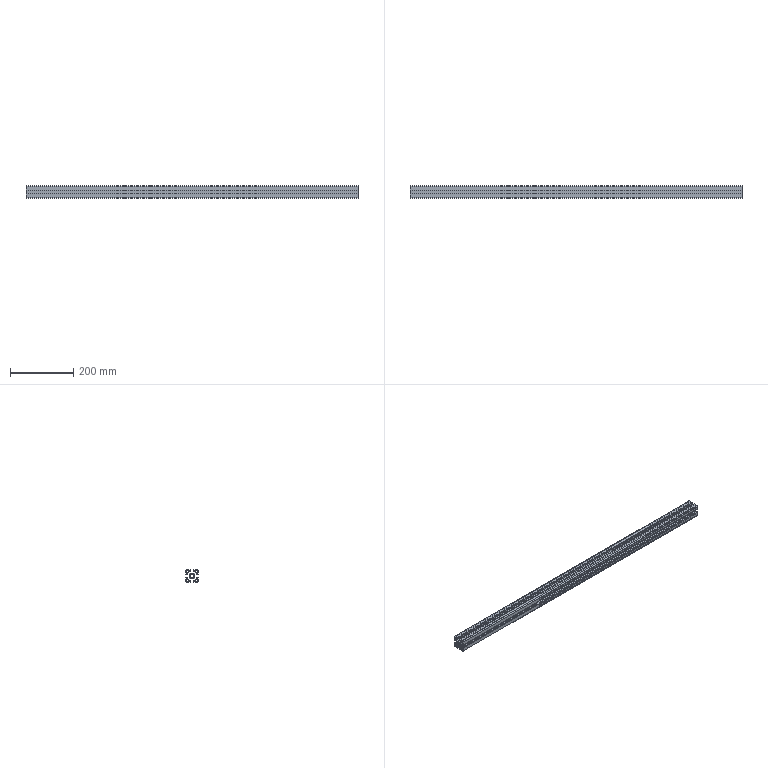Part | STEP file | AL PROFILE 4040 L 900 | 1 solid | 137 faces | box 1050 x 40 x 40 mm | volume 583573 mm3 | plane 110 | cylinder 27 | commonest cylinder face diameters 3 x10 5.5 x8 10 x5 6 x4